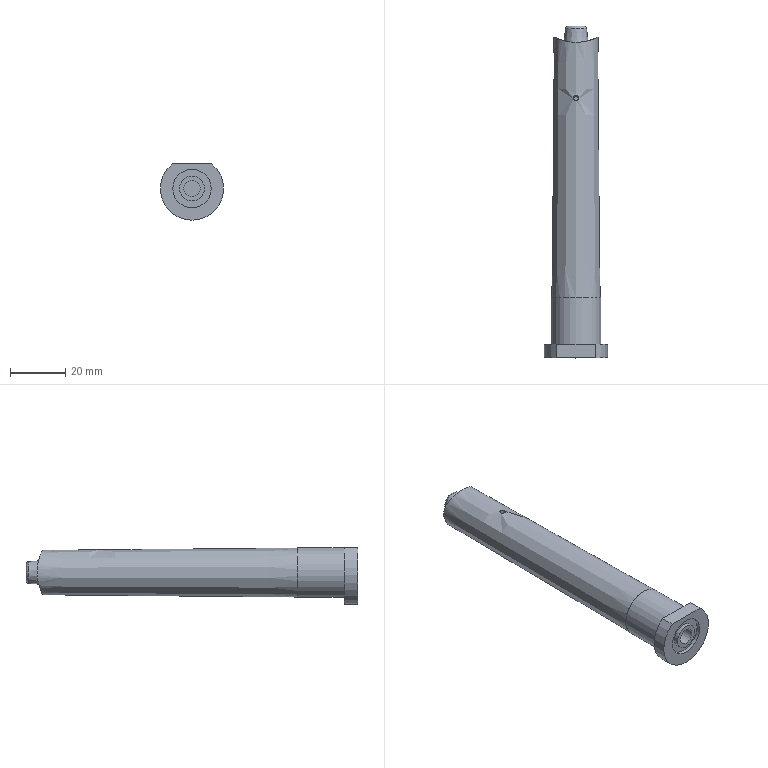Part | NX | features solid 2 | 1 solid | 19 faces | box 23 x 120.548 x 20.5 mm | volume 24480 mm3 | plane 9 | cylinder 5 | cone 4 | torus 1 | commonest cylinder face diameters 6 x1 9 x1 14 x1 18 x1 23 x1
STEP:
#1=CARTESIAN_POINT('',(7.,-132.,8.725));
#2=VERTEX_POINT('',#1);
#3=CARTESIAN_POINT('',(0.,-132.,8.725));
#4=DIRECTION('',(0.,1.,0.));
#5=DIRECTION('',(1.,0.,0.));
#6=AXIS2_PLACEMENT_3D('',#3,#4,#5);
#7=CIRCLE('',#6,7.);
#8=EDGE_CURVE('',#2,#2,#7,.T.);
#9=ORIENTED_EDGE('',*,*,#8,.T.);
#10=EDGE_LOOP('',(#9));
#11=FACE_BOUND('',#10,.T.);
#12=CARTESIAN_POINT('',(7.159,-132.,17.725));
#13=VERTEX_POINT('',#12);
#14=CARTESIAN_POINT('',(-7.159,-132.,17.725));
#15=VERTEX_POINT('',#14);
#16=CARTESIAN_POINT('',(0.,-132.,8.725));
#17=DIRECTION('',(0.,-1.,0.));
#18=DIRECTION('',(0.,0.,-1.));
#19=AXIS2_PLACEMENT_3D('',#16,#17,#18);
#20=CIRCLE('',#19,11.5);
#21=EDGE_CURVE('',#13,#15,#20,.F.);
#22=ORIENTED_EDGE('',*,*,#21,.F.);
#23=CARTESIAN_POINT('',(0.,-132.,17.725));
#24=DIRECTION('',(-1.,0.,0.));
#25=VECTOR('',#24,1000.);
#26=LINE('',#23,#25);
#27=EDGE_CURVE('',#15,#13,#26,.F.);
#28=ORIENTED_EDGE('',*,*,#27,.F.);
#29=EDGE_LOOP('',(#22,#28));
#30=FACE_BOUND('',#29,.T.);
#31=CARTESIAN_POINT('',(0.,-132.,-5.275));
#32=DIRECTION('',(0.,-1.,0.));
#33=DIRECTION('',(0.,0.,1.));
#34=AXIS2_PLACEMENT_3D('',#31,#32,#33);
#35=PLANE('',#34);
#36=ADVANCED_FACE('',(#11,#30),#35,.T.);
#37=ORIENTED_EDGE('',*,*,#21,.T.);
#38=CARTESIAN_POINT('',(-7.159,-127.,17.725));
#39=VERTEX_POINT('',#38);
#40=CARTESIAN_POINT('',(-7.159,-124.,17.725));
#41=DIRECTION('',(0.,-1.,0.));
#42=VECTOR('',#41,1000.);
#43=LINE('',#40,#42);
#44=EDGE_CURVE('',#15,#39,#43,.F.);
#45=ORIENTED_EDGE('',*,*,#44,.T.);
#46=CARTESIAN_POINT('',(7.159,-127.,17.725));
#47=VERTEX_POINT('',#46);
#48=CARTESIAN_POINT('',(0.,-127.,8.725));
#49=DIRECTION('',(0.,-1.,0.));
#50=DIRECTION('',(0.,0.,-1.));
#51=AXIS2_PLACEMENT_3D('',#48,#49,#50);
#52=CIRCLE('',#51,11.5);
#53=EDGE_CURVE('',#47,#39,#52,.F.);
#54=ORIENTED_EDGE('',*,*,#53,.F.);
#55=CARTESIAN_POINT('',(7.159,-124.,17.725));
#56=DIRECTION('',(0.,-1.,0.));
#57=VECTOR('',#56,1000.);
#58=LINE('',#55,#57);
#59=EDGE_CURVE('',#47,#13,#58,.T.);
#60=ORIENTED_EDGE('',*,*,#59,.T.);
#61=EDGE_LOOP('',(#37,#45,#54,#60));
#62=FACE_BOUND('',#61,.T.);
#63=CARTESIAN_POINT('',(0.,-124.,8.725));
#64=DIRECTION('',(0.,-1.,0.));
#65=DIRECTION('',(0.,0.,1.));
#66=AXIS2_PLACEMENT_3D('',#63,#64,#65);
#67=CYLINDRICAL_SURFACE('',#66,11.5);
#68=ADVANCED_FACE('',(#62),#67,.T.);
#69=CARTESIAN_POINT('',(0.,-127.,17.725));
#70=VERTEX_POINT('',#69);
#71=CARTESIAN_POINT('',(0.,-127.,17.725));
#72=DIRECTION('',(-1.,0.,0.));
#73=VECTOR('',#72,1000.);
#74=LINE('',#71,#73);
#75=EDGE_CURVE('',#70,#47,#74,.F.);
#76=ORIENTED_EDGE('',*,*,#75,.T.);
#77=ORIENTED_EDGE('',*,*,#53,.T.);
#78=CARTESIAN_POINT('',(0.,-127.,17.725));
#79=DIRECTION('',(-1.,0.,0.));
#80=VECTOR('',#79,1000.);
#81=LINE('',#78,#80);
#82=EDGE_CURVE('',#39,#70,#81,.F.);
#83=ORIENTED_EDGE('',*,*,#82,.T.);
#84=CARTESIAN_POINT('',(0.,-127.,8.725));
#85=DIRECTION('',(0.,-1.,0.));
#86=DIRECTION('',(0.,0.,-1.));
#87=AXIS2_PLACEMENT_3D('',#84,#85,#86);
#88=CIRCLE('',#87,9.);
#89=EDGE_CURVE('',#70,#70,#88,.T.);
#90=ORIENTED_EDGE('',*,*,#89,.T.);
#91=EDGE_LOOP('',(#76,#77,#83,#90));
#92=FACE_BOUND('',#91,.T.);
#93=CARTESIAN_POINT('',(0.,-127.,8.725));
#94=DIRECTION('',(0.,-1.,0.));
#95=DIRECTION('',(0.,0.,1.));
#96=AXIS2_PLACEMENT_3D('',#93,#94,#95);
#97=PLANE('',#96);
#98=ADVANCED_FACE('',(#92),#97,.F.);
#99=CARTESIAN_POINT('',(0.,-110.,17.614));
#100=VERTEX_POINT('',#99);
#101=CARTESIAN_POINT('',(0.,-110.,8.725));
#102=DIRECTION('',(0.,1.,0.));
#103=DIRECTION('',(0.,0.,1.));
#104=AXIS2_PLACEMENT_3D('',#101,#102,#103);
#105=CIRCLE('',#104,8.889);
#106=EDGE_CURVE('',#100,#100,#105,.T.);
#107=ORIENTED_EDGE('',*,*,#106,.F.);
#108=EDGE_LOOP('',(#107));
#109=FACE_BOUND('',#108,.T.);
#110=CARTESIAN_POINT('',(0.,-110.,17.725));
#111=VERTEX_POINT('',#110);
#112=CARTESIAN_POINT('',(0.,-110.,8.725));
#113=DIRECTION('',(0.,1.,0.));
#114=DIRECTION('',(0.,0.,1.));
#115=AXIS2_PLACEMENT_3D('',#112,#113,#114);
#116=CIRCLE('',#115,9.);
#117=EDGE_CURVE('',#111,#111,#116,.T.);
#118=ORIENTED_EDGE('',*,*,#117,.T.);
#119=EDGE_LOOP('',(#118));
#120=FACE_BOUND('',#119,.T.);
#121=CARTESIAN_POINT('',(0.,-110.,8.725));
#122=DIRECTION('',(0.,1.,0.));
#123=DIRECTION('',(0.,0.,-1.));
#124=AXIS2_PLACEMENT_3D('',#121,#122,#123);
#125=PLANE('',#124);
#126=ADVANCED_FACE('',(#109,#120),#125,.T.);
#127=ORIENTED_EDGE('',*,*,#89,.F.);
#128=EDGE_LOOP('',(#127));
#129=FACE_BOUND('',#128,.T.);
#130=ORIENTED_EDGE('',*,*,#117,.F.);
#131=EDGE_LOOP('',(#130));
#132=FACE_BOUND('',#131,.T.);
#133=CARTESIAN_POINT('',(0.,-205.,8.725));
#134=DIRECTION('',(0.,1.,0.));
#135=DIRECTION('',(0.,0.,1.));
#136=AXIS2_PLACEMENT_3D('',#133,#134,#135);
#137=CYLINDRICAL_SURFACE('',#136,9.);
#138=ADVANCED_FACE('',(#129,#132),#137,.T.);
#139=CARTESIAN_POINT('',(0.,-17.5,0.6439));
#140=VERTEX_POINT('',#139);
#141=CARTESIAN_POINT('',(-3.216,-17.288,1.085));
#142=CARTESIAN_POINT('',(0.0006962,-17.606,0.4238));
#143=CARTESIAN_POINT('',(3.213,-17.288,1.084));
#144=CARTESIAN_POINT('',(5.85,-16.53,2.874));
#145=CARTESIAN_POINT('',(7.619,-15.726,5.502));
#146=CARTESIAN_POINT('',(8.281,-15.334,8.693));
#147=CARTESIAN_POINT('',(7.636,-15.655,11.92));
#148=CARTESIAN_POINT('',(5.858,-16.419,14.569));
#149=CARTESIAN_POINT('',(3.221,-17.151,16.362));
#150=CARTESIAN_POINT('',(0.01839,-17.462,17.024));
#151=CARTESIAN_POINT('',(-3.199,-17.156,16.373));
#152=CARTESIAN_POINT('',(-5.852,-16.421,14.576));
#153=CARTESIAN_POINT('',(-7.628,-15.659,11.933));
#154=CARTESIAN_POINT('',(-8.281,-15.333,8.727));
#155=CARTESIAN_POINT('',(-7.629,-15.721,5.519));
#156=CARTESIAN_POINT('',(-5.852,-16.529,2.876));
#157=CARTESIAN_POINT('',(-3.216,-17.288,1.085));
#158=CARTESIAN_POINT('',(0.0006962,-17.606,0.4238));
#159=CARTESIAN_POINT('',(3.213,-17.288,1.084));
#160=B_SPLINE_CURVE_WITH_KNOTS('',3,(#141,#142,#143,#144,#145,#146,#147,#148,#149,#150,#151,#152,#153,#154,#155,#156,#157,#158,#159),.UNSPECIFIED.,.T.,.F.,(1,1,1,1,1,1,1,1,1,1,1,1,1,1,1,1,1,1,1,1,1,1,1),(-0.009597,-0.006398,-0.003199,0.,0.003199,0.006398,0.009597,0.0128,0.016,0.01919,0.02239,0.02559,0.02879,0.03199,0.03519,0.03839,0.04159,0.04479,0.04799,0.05118,0.05438,0.05758,0.06078),.UNSPECIFIED.);
#161=EDGE_CURVE('',#140,#140,#160,.T.);
#162=ORIENTED_EDGE('',*,*,#161,.F.);
#163=EDGE_LOOP('',(#162));
#164=FACE_BOUND('',#163,.T.);
#165=CARTESIAN_POINT('',(-3.148,-17.17,5.715));
#166=VERTEX_POINT('',#165);
#167=CARTESIAN_POINT('',(-0.1207,-17.607,3.863));
#168=CARTESIAN_POINT('',(-3.495,-17.166,5.395));
#169=CARTESIAN_POINT('',(-4.79,-16.745,8.843));
#170=CARTESIAN_POINT('',(-3.323,-17.147,12.223));
#171=CARTESIAN_POINT('',(0.1224,-17.523,13.581));
#172=CARTESIAN_POINT('',(3.495,-17.107,12.048));
#173=CARTESIAN_POINT('',(4.79,-16.747,8.598));
#174=CARTESIAN_POINT('',(3.32,-17.21,5.218));
#175=CARTESIAN_POINT('',(-0.1207,-17.607,3.863));
#176=CARTESIAN_POINT('',(-3.495,-17.166,5.395));
#177=CARTESIAN_POINT('',(-4.79,-16.745,8.843));
#178=B_SPLINE_CURVE_WITH_KNOTS('',3,(#167,#168,#169,#170,#171,#172,#173,#174,#175,#176,#177),.UNSPECIFIED.,.T.,.F.,(1,1,1,1,1,1,1,1,1,1,1,1,1,1,1),(-0.01025,-0.006833,-0.003417,0.,0.003417,0.006833,0.01025,0.01367,0.01708,0.0205,0.02392,0.02733,0.03075,0.03417,0.03758),.UNSPECIFIED.);
#179=EDGE_CURVE('',#166,#166,#178,.T.);
#180=ORIENTED_EDGE('',*,*,#179,.F.);
#181=EDGE_LOOP('',(#180));
#182=FACE_BOUND('',#181,.T.);
#183=CARTESIAN_POINT('',(0.,0.,4.707));
#184=DIRECTION('',(0.,0.,-1.));
#185=DIRECTION('',(1.,0.,0.));
#186=AXIS2_PLACEMENT_3D('',#183,#184,#185);
#187=CONICAL_SURFACE('',#186,17.465,0.008727);
#188=ADVANCED_FACE('',(#164,#182),#187,.F.);
#189=ORIENTED_EDGE('',*,*,#161,.T.);
#190=EDGE_LOOP('',(#189));
#191=FACE_BOUND('',#190,.T.);
#192=ORIENTED_EDGE('',*,*,#106,.T.);
#193=EDGE_LOOP('',(#192));
#194=FACE_BOUND('',#193,.T.);
#195=CARTESIAN_POINT('',(0.8766,-37.292,16.933));
#196=VERTEX_POINT('',#195);
#197=CARTESIAN_POINT('',(0.3775,-36.688,16.977));
#198=CARTESIAN_POINT('',(0.9717,-37.25,16.923));
#199=CARTESIAN_POINT('',(0.9956,-38.066,16.926));
#200=CARTESIAN_POINT('',(0.4399,-38.661,16.991));
#201=CARTESIAN_POINT('',(-0.3781,-38.687,16.995));
#202=CARTESIAN_POINT('',(-0.9707,-38.127,16.931));
#203=CARTESIAN_POINT('',(-0.9966,-37.312,16.92));
#204=CARTESIAN_POINT('',(-0.4401,-36.714,16.974));
#205=CARTESIAN_POINT('',(0.3775,-36.688,16.977));
#206=CARTESIAN_POINT('',(0.9717,-37.25,16.923));
#207=CARTESIAN_POINT('',(0.9956,-38.066,16.926));
#208=B_SPLINE_CURVE_WITH_KNOTS('',3,(#197,#198,#199,#200,#201,#202,#203,#204,#205,#206,#207),.UNSPECIFIED.,.T.,.F.,(1,1,1,1,1,1,1,1,1,1,1,1,1,1,1),(-0.002259,-0.001506,-0.0007531,0.,0.0007531,0.001506,0.002259,0.003012,0.003765,0.004518,0.005272,0.006025,0.006778,0.007531,0.008284),.UNSPECIFIED.);
#209=EDGE_CURVE('',#196,#196,#208,.T.);
#210=ORIENTED_EDGE('',*,*,#209,.T.);
#211=EDGE_LOOP('',(#210));
#212=FACE_BOUND('',#211,.T.);
#213=CARTESIAN_POINT('',(0.,-42.901,8.725));
#214=DIRECTION('',(0.,-1.,0.));
#215=DIRECTION('',(0.,0.,1.));
#216=AXIS2_PLACEMENT_3D('',#213,#214,#215);
#217=CONICAL_SURFACE('',#216,8.303,0.008727);
#218=ADVANCED_FACE('',(#191,#194,#212),#217,.T.);
#219=CARTESIAN_POINT('',(0.,-12.364,4.79));
#220=VERTEX_POINT('',#219);
#221=CARTESIAN_POINT('',(0.,-12.364,8.725));
#222=DIRECTION('',(0.,-1.,0.));
#223=DIRECTION('',(0.,0.,-1.));
#224=AXIS2_PLACEMENT_3D('',#221,#222,#223);
#225=CIRCLE('',#224,3.936);
#226=EDGE_CURVE('',#220,#220,#225,.T.);
#227=ORIENTED_EDGE('',*,*,#226,.T.);
#228=EDGE_LOOP('',(#227));
#229=FACE_BOUND('',#228,.T.);
#230=ORIENTED_EDGE('',*,*,#179,.T.);
#231=EDGE_LOOP('',(#230));
#232=FACE_BOUND('',#231,.T.);
#233=CARTESIAN_POINT('',(0.,-13.8,8.725));
#234=DIRECTION('',(0.,-1.,0.));
#235=DIRECTION('',(0.,0.,1.));
#236=AXIS2_PLACEMENT_3D('',#233,#234,#235);
#237=CONICAL_SURFACE('',#236,4.061,0.08727);
#238=ADVANCED_FACE('',(#229,#232),#237,.T.);
#239=CARTESIAN_POINT('',(0.,-11.452,11.665));
#240=VERTEX_POINT('',#239);
#241=CARTESIAN_POINT('',(0.,-11.452,8.725));
#242=DIRECTION('',(0.,1.,0.));
#243=DIRECTION('',(0.,0.,1.));
#244=AXIS2_PLACEMENT_3D('',#241,#242,#243);
#245=CIRCLE('',#244,2.939);
#246=EDGE_CURVE('',#240,#240,#245,.T.);
#247=ORIENTED_EDGE('',*,*,#246,.T.);
#248=EDGE_LOOP('',(#247));
#249=FACE_BOUND('',#248,.T.);
#250=CARTESIAN_POINT('',(0.,-11.452,8.725));
#251=DIRECTION('',(0.,1.,0.));
#252=DIRECTION('',(0.,0.,1.));
#253=AXIS2_PLACEMENT_3D('',#250,#251,#252);
#254=PLANE('',#253);
#255=ADVANCED_FACE('',(#249),#254,.T.);
#256=ORIENTED_EDGE('',*,*,#226,.F.);
#257=EDGE_LOOP('',(#256));
#258=FACE_BOUND('',#257,.T.);
#259=ORIENTED_EDGE('',*,*,#246,.F.);
#260=EDGE_LOOP('',(#259));
#261=FACE_BOUND('',#260,.T.);
#262=CARTESIAN_POINT('',(0.,-12.452,8.725));
#263=DIRECTION('',(0.,1.,0.));
#264=DIRECTION('',(0.,0.,1.));
#265=AXIS2_PLACEMENT_3D('',#262,#263,#264);
#266=TOROIDAL_SURFACE('',#265,2.939,1.);
#267=ADVANCED_FACE('',(#258,#261),#266,.T.);
#268=CARTESIAN_POINT('',(-0.8046,-37.688,13.936));
#269=VERTEX_POINT('',#268);
#270=CARTESIAN_POINT('',(0.,-37.688,13.936));
#271=DIRECTION('',(0.,0.,-1.));
#272=DIRECTION('',(-1.,0.,0.));
#273=AXIS2_PLACEMENT_3D('',#270,#271,#272);
#274=CIRCLE('',#273,0.8046);
#275=EDGE_CURVE('',#269,#269,#274,.T.);
#276=ORIENTED_EDGE('',*,*,#275,.F.);
#277=EDGE_LOOP('',(#276));
#278=FACE_BOUND('',#277,.T.);
#279=CARTESIAN_POINT('',(0.,-37.688,13.936));
#280=DIRECTION('',(0.,0.,-1.));
#281=DIRECTION('',(-1.,0.,0.));
#282=AXIS2_PLACEMENT_3D('',#279,#280,#281);
#283=PLANE('',#282);
#284=ADVANCED_FACE('',(#278),#283,.F.);
#285=ORIENTED_EDGE('',*,*,#275,.T.);
#286=EDGE_LOOP('',(#285));
#287=FACE_BOUND('',#286,.T.);
#288=ORIENTED_EDGE('',*,*,#209,.F.);
#289=EDGE_LOOP('',(#288));
#290=FACE_BOUND('',#289,.T.);
#291=CARTESIAN_POINT('',(0.,-37.688,14.236));
#292=DIRECTION('',(0.,0.,1.));
#293=DIRECTION('',(-1.,0.,0.));
#294=AXIS2_PLACEMENT_3D('',#291,#292,#293);
#295=CONICAL_SURFACE('',#294,0.8203,0.05236);
#296=ADVANCED_FACE('',(#287,#290),#295,.F.);
#297=CARTESIAN_POINT('',(7.,-130.6,8.725));
#298=VERTEX_POINT('',#297);
#299=CARTESIAN_POINT('',(0.,-130.6,8.725));
#300=DIRECTION('',(0.,-1.,0.));
#301=DIRECTION('',(1.,0.,0.));
#302=AXIS2_PLACEMENT_3D('',#299,#300,#301);
#303=CIRCLE('',#302,7.);
#304=EDGE_CURVE('',#298,#298,#303,.F.);
#305=ORIENTED_EDGE('',*,*,#304,.F.);
#306=EDGE_LOOP('',(#305));
#307=FACE_BOUND('',#306,.T.);
#308=CARTESIAN_POINT('',(4.5,-130.6,8.725));
#309=VERTEX_POINT('',#308);
#310=CARTESIAN_POINT('',(0.,-130.6,8.725));
#311=DIRECTION('',(0.,-1.,0.));
#312=DIRECTION('',(1.,0.,0.));
#313=AXIS2_PLACEMENT_3D('',#310,#311,#312);
#314=CIRCLE('',#313,4.5);
#315=EDGE_CURVE('',#309,#309,#314,.F.);
#316=ORIENTED_EDGE('',*,*,#315,.T.);
#317=EDGE_LOOP('',(#316));
#318=FACE_BOUND('',#317,.T.);
#319=CARTESIAN_POINT('',(0.,-130.6,8.725));
#320=DIRECTION('',(0.,1.,0.));
#321=DIRECTION('',(0.,0.,1.));
#322=AXIS2_PLACEMENT_3D('',#319,#320,#321);
#323=PLANE('',#322);
#324=ADVANCED_FACE('',(#307,#318),#323,.F.);
#325=ORIENTED_EDGE('',*,*,#304,.T.);
#326=EDGE_LOOP('',(#325));
#327=FACE_BOUND('',#326,.T.);
#328=ORIENTED_EDGE('',*,*,#8,.F.);
#329=EDGE_LOOP('',(#328));
#330=FACE_BOUND('',#329,.T.);
#331=CARTESIAN_POINT('',(0.,-132.,8.725));
#332=DIRECTION('',(0.,1.,0.));
#333=DIRECTION('',(1.,0.,0.));
#334=AXIS2_PLACEMENT_3D('',#331,#332,#333);
#335=CYLINDRICAL_SURFACE('',#334,7.);
#336=ADVANCED_FACE('',(#327,#330),#335,.F.);
#337=ORIENTED_EDGE('',*,*,#315,.F.);
#338=EDGE_LOOP('',(#337));
#339=FACE_BOUND('',#338,.T.);
#340=CARTESIAN_POINT('',(4.5,-132.,8.725));
#341=VERTEX_POINT('',#340);
#342=CARTESIAN_POINT('',(0.,-132.,8.725));
#343=DIRECTION('',(0.,1.,0.));
#344=DIRECTION('',(1.,0.,0.));
#345=AXIS2_PLACEMENT_3D('',#342,#343,#344);
#346=CIRCLE('',#345,4.5);
#347=EDGE_CURVE('',#341,#341,#346,.T.);
#348=ORIENTED_EDGE('',*,*,#347,.T.);
#349=EDGE_LOOP('',(#348));
#350=FACE_BOUND('',#349,.T.);
#351=CARTESIAN_POINT('',(0.,-132.,8.725));
#352=DIRECTION('',(0.,1.,0.));
#353=DIRECTION('',(1.,0.,0.));
#354=AXIS2_PLACEMENT_3D('',#351,#352,#353);
#355=CYLINDRICAL_SURFACE('',#354,4.5);
#356=ADVANCED_FACE('',(#339,#350),#355,.T.);
#357=CARTESIAN_POINT('',(0.,-25.,5.725));
#358=VERTEX_POINT('',#357);
#359=CARTESIAN_POINT('',(0.,-25.,8.725));
#360=DIRECTION('',(0.,-1.,0.));
#361=DIRECTION('',(0.,0.,-1.));
#362=AXIS2_PLACEMENT_3D('',#359,#360,#361);
#363=CIRCLE('',#362,3.);
#364=EDGE_CURVE('',#358,#358,#363,.F.);
#365=ORIENTED_EDGE('',*,*,#364,.F.);
#366=EDGE_LOOP('',(#365));
#367=FACE_BOUND('',#366,.T.);
#368=CARTESIAN_POINT('',(0.,-25.,8.725));
#369=DIRECTION('',(0.,-1.,0.));
#370=DIRECTION('',(0.,0.,-1.));
#371=AXIS2_PLACEMENT_3D('',#368,#369,#370);
#372=PLANE('',#371);
#373=ADVANCED_FACE('',(#367),#372,.T.);
#374=CARTESIAN_POINT('',(0.,-132.,5.725));
#375=VERTEX_POINT('',#374);
#376=CARTESIAN_POINT('',(0.,-132.,8.725));
#377=DIRECTION('',(0.,-1.,0.));
#378=DIRECTION('',(0.,0.,-1.));
#379=AXIS2_PLACEMENT_3D('',#376,#377,#378);
#380=CIRCLE('',#379,3.);
#381=EDGE_CURVE('',#375,#375,#380,.T.);
#382=ORIENTED_EDGE('',*,*,#381,.T.);
#383=EDGE_LOOP('',(#382));
#384=FACE_BOUND('',#383,.T.);
#385=ORIENTED_EDGE('',*,*,#364,.T.);
#386=EDGE_LOOP('',(#385));
#387=FACE_BOUND('',#386,.T.);
#388=CARTESIAN_POINT('',(0.,-29.,8.725));
#389=DIRECTION('',(0.,-1.,0.));
#390=DIRECTION('',(0.,0.,-1.));
#391=AXIS2_PLACEMENT_3D('',#388,#389,#390);
#392=CYLINDRICAL_SURFACE('',#391,3.);
#393=ADVANCED_FACE('',(#384,#387),#392,.F.);
#394=ORIENTED_EDGE('',*,*,#347,.F.);
#395=EDGE_LOOP('',(#394));
#396=FACE_BOUND('',#395,.T.);
#397=ORIENTED_EDGE('',*,*,#381,.F.);
#398=EDGE_LOOP('',(#397));
#399=FACE_BOUND('',#398,.T.);
#400=CARTESIAN_POINT('',(0.,-132.,-5.275));
#401=DIRECTION('',(0.,-1.,0.));
#402=DIRECTION('',(0.,0.,1.));
#403=AXIS2_PLACEMENT_3D('',#400,#401,#402);
#404=PLANE('',#403);
#405=ADVANCED_FACE('',(#396,#399),#404,.T.);
#406=ORIENTED_EDGE('',*,*,#59,.F.);
#407=ORIENTED_EDGE('',*,*,#75,.F.);
#408=ORIENTED_EDGE('',*,*,#82,.F.);
#409=ORIENTED_EDGE('',*,*,#44,.F.);
#410=ORIENTED_EDGE('',*,*,#27,.T.);
#411=EDGE_LOOP('',(#406,#407,#408,#409,#410));
#412=FACE_BOUND('',#411,.T.);
#413=CARTESIAN_POINT('',(0.,-127.,17.725));
#414=DIRECTION('',(0.,0.,1.));
#415=DIRECTION('',(1.,0.,0.));
#416=AXIS2_PLACEMENT_3D('',#413,#414,#415);
#417=PLANE('',#416);
#418=ADVANCED_FACE('',(#412),#417,.T.);
#419=CLOSED_SHELL('',(#36,#68,#98,#126,#138,#188,#218,#238,#255,#267,#284,#296,#324,#336,#356,#373,#393,#405,#418));
#420=MANIFOLD_SOLID_BREP('',#419);
#421=(LENGTH_UNIT()NAMED_UNIT(*)SI_UNIT(.MILLI.,.METRE.));
#422=UNCERTAINTY_MEASURE_WITH_UNIT(LENGTH_MEASURE(0.0508),#421,'','');
#423=(NAMED_UNIT(*)PLANE_ANGLE_UNIT()SI_UNIT($,.RADIAN.));
#424=(NAMED_UNIT(*)SI_UNIT($,.STERADIAN.)SOLID_ANGLE_UNIT());
#425=(GEOMETRIC_REPRESENTATION_CONTEXT(3)GLOBAL_UNCERTAINTY_ASSIGNED_CONTEXT((#422))GLOBAL_UNIT_ASSIGNED_CONTEXT((#421,#423,#424))REPRESENTATION_CONTEXT('',''));
#426=ADVANCED_BREP_SHAPE_REPRESENTATION('',(#420),#425);